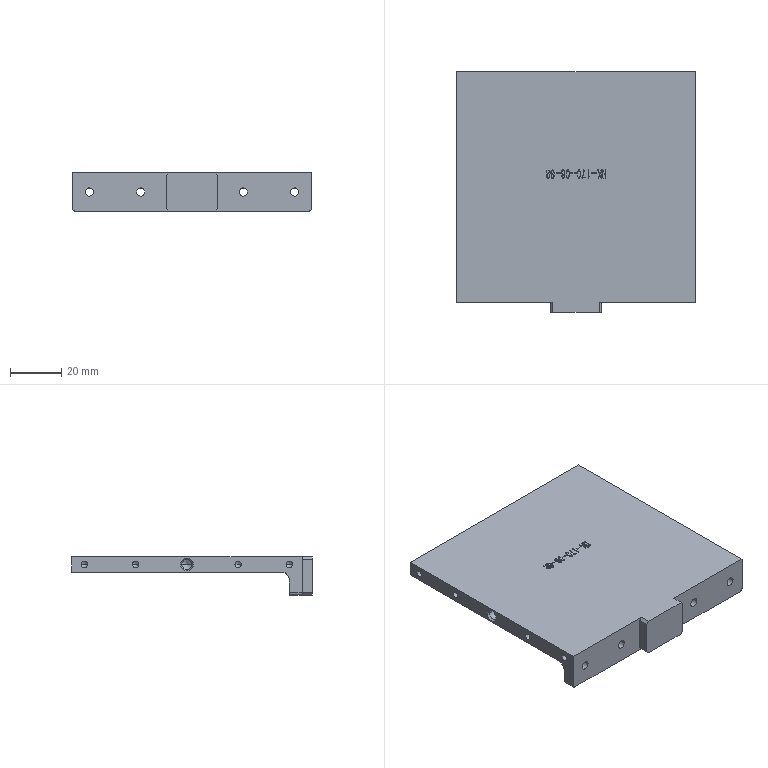NC program | NX | posted with a generic post | part box 93.2 x 94 x 15 mm
Whole program:
N10 G17 G21 G94 G90
(DRILLING_COPY_COPY , TOOL : D6A45)
N12 T01 M6
N14 G54
N16 G17 G0 G90 X-38. Y3. B0. C0. S5000 M3
N18 G43 Z30. H1
N20 G94 G81 G98 Z-1.6 F350. R3.
N22 X-18.
N24 X2.
N26 X22.
N28 X42.
N30 G80
N32 G0 X42. Y3. Z30.
N34 M5
(DRILLING_COPY_1_COPY_COPY , TOOL : 2.5ZT)
N36 T02 M6
N38 G54
N40 G17 G0 G90 X-38. Y3. B0. C0. S2000 M3
N42 G43 Z30. H2
N44 G94 G83 G98 Z-9.251 F200. Q2. R3.
N46 X-18.
N48 X22.
N50 X42.
N52 G80
N54 G0 X42. Y3. Z30.
N56 M5
(HOLE_MILLING , TOOL : D3)
N58 T17 M6
N60 G54
N62 G17 G0 G90 X2. Y3. B0. C0. S9500 M3
N64 G43 Z30. H17
N66 Z0.5
N68 G94 G3 X2.2 Y2.8 R0.2 F1000.
N70 X2.4 Y3. R0.2
N72 X2.4 Y3. Z0.3 I-0.4 J0.
N74 X2.4 Y3. Z0.1 I-0.4 J0.
N76 X2.4 Y3. Z-0.1 I-0.4 J0.
N78 X2.4 Y3. Z-0.3 I-0.4 J0.
N80 X2.4 Y3. Z-0.5 I-0.4 J0.
N82 X2.4 Y3. Z-0.7 I-0.4 J0.
N84 X2.4 Y3. Z-0.9 I-0.4 J0.
N86 X2.4 Y3. Z-1.1 I-0.4 J0.
N88 X2.4 Y3. Z-1.3 I-0.4 J0.
N90 X2.4 Y3. Z-1.5 I-0.4 J0.
N92 X2.4 Y3. Z-1.7 I-0.4 J0.
N94 X2.4 Y3. Z-1.9 I-0.4 J0.
N96 X2.4 Y3. Z-2.1 I-0.4 J0.
N98 X2.4 Y3. Z-2.3 I-0.4 J0.
N100 X2.4 Y3. Z-2.5 I-0.4 J0.
N102 X2.4 Y3. Z-2.7 I-0.4 J0.
N104 X2.4 Y3. Z-2.9 I-0.4 J0.
N106 X2.4 Y3. Z-3.1 I-0.4 J0.
N108 X2.4 Y3. Z-3.3 I-0.4 J0.
N110 X2.4 Y3. Z-3.5 I-0.4 J0.
N112 X2.4 Y3. Z-3.7 I-0.4 J0.
N114 X2.4 Y3. Z-3.9 I-0.4 J0.
N116 X2.4 Y3. Z-4.1 I-0.4 J0.
N118 X2.4 Y3. Z-4.3 I-0.4 J0.
N120 X2.4 Y3. Z-4.5 I-0.4 J0.
N122 X2.4 Y3. Z-4.7 I-0.4 J0.
N124 X2.4 Y3. Z-4.9 I-0.4 J0.
N126 X2.4 Y3. Z-5.1 I-0.4 J0.
N128 X2.4 Y3. Z-5.3 I-0.4 J0.
N130 X2.4 Y3. Z-5.5 I-0.4 J0.
N132 X2.4 Y3. Z-5.7 I-0.4 J0.
N134 X2.4 Y3. Z-5.9 I-0.4 J0.
N136 X2.4 Y3. Z-6.1 I-0.4 J0.
N138 X2.4 Y3. Z-6.3 I-0.4 J0.
N140 X2.4 Y3. Z-6.5 I-0.4 J0.
N142 X2.4 Y3. Z-6.7 I-0.4 J0.
N144 X2.4 Y3. Z-6.9 I-0.4 J0.
N146 X2.4 Y3. Z-7.1 I-0.4 J0.
N148 X2.4 Y3. Z-7.3 I-0.4 J0.
N150 X2.4 Y3. Z-7.5 I-0.4 J0.
N152 X2.4 Y3. Z-7.7 I-0.4 J0.
N154 X2.4 Y3. Z-7.9 I-0.4 J0.
N156 X2.4 Y3. Z-8.1 I-0.4 J0.
N158 X2.4 Y3. Z-8.3 I-0.4 J0.
N160 X2.4 Y3. Z-8.5 I-0.4 J0.
N162 X2. Y3.4 R0.4
N164 X2.4 Y3. R-0.4
N166 X2.2 Y3.2 R0.2
N168 X2. Y3. R0.2
N170 G0 Z30.
N172 M5
(DRILLING_COPY_COPY_COPY , TOOL : D6A45)
N174 T01 M6
N176 G54
N178 G17 G0 G90 X2. Y3. B0. C0. S5000 M3
N180 G43 Z30. H1
N182 G94 G81 G98 Z-2.5 F350. R3.
N184 G80
N186 G0 X2. Y3. Z30.
N188 M5
(HOLE_MILLING_COPY , TOOL : D3)
N190 T17 M6
N192 G54
N194 G17 G0 G90 X2. Y3. B0. C0. S9500 M3
N196 G43 Z30. H17
N198 Z0.5
N200 G41 G94 G1 X2.027 Y2.904 F1000. D17
N202 G3 X2.45 Y3. R0.222
N204 X2.45 Y3. Z-1.5 I-0.45 J0.
N206 X2.45 Y3. Z-3.5 I-0.45 J0.
N208 X2.45 Y3. Z-5.5 I-0.45 J0.
N210 X2.45 Y3. Z-7.5 I-0.45 J0.
N212 X1.55 Y3. Z-8.5 I-0.45 J0.
N214 X2. Y2.55 R0.45
N216 X1.55 Y3. R-0.45
N218 X1.973 Y2.904 R0.222
N220 G40
N222 G1 X2. Y3.
N224 G0 Z30.
N226 M5
N228 M2